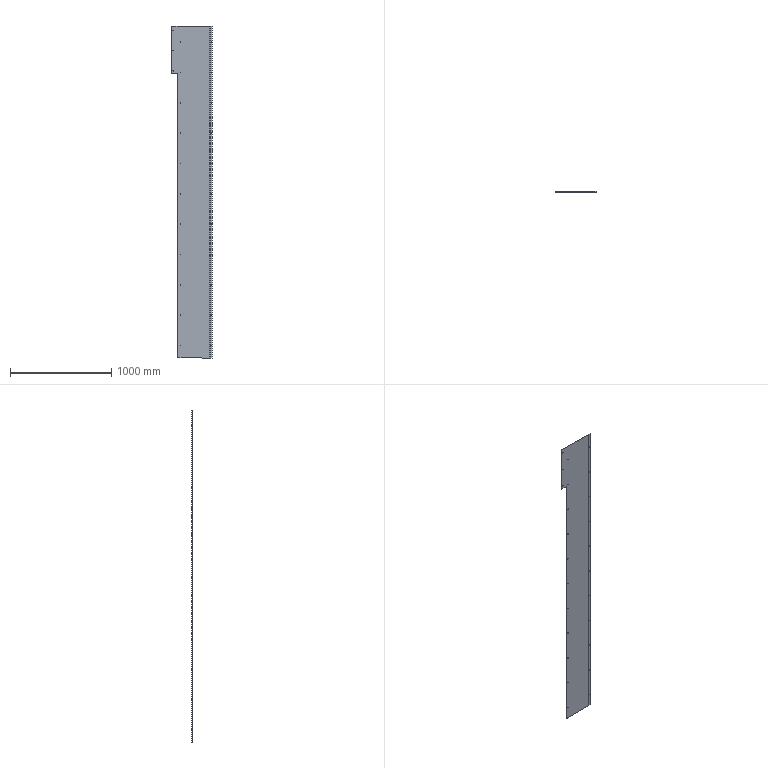Part | STEP file | TS-S35 | 1 solid | 76 faces | box 398 x 4.2 x 3283 mm | volume 1369495 mm3 | cylinder 55 | plane 21 | commonest cylinder face diameters 5.4 x50 0.4 x2 2.8 x2 10 x1